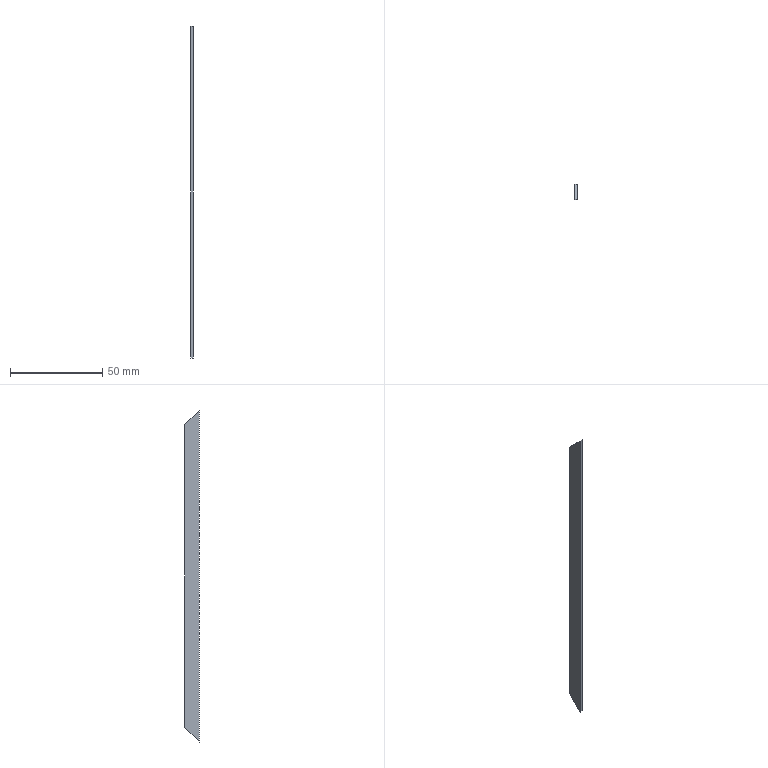Part | NX | features BREP 1 | 1 solid | 6 faces | box 1.5 x 8 x 179.5 mm | volume 2058 mm3 | plane 6
STEP:
#1=CARTESIAN_POINT('',(0.,8.,81.75));
#2=VERTEX_POINT('',#1);
#3=CARTESIAN_POINT('',(0.,8.,-81.75));
#4=VERTEX_POINT('',#3);
#5=CARTESIAN_POINT('',(0.,8.,89.75));
#6=DIRECTION('',(0.,0.,-1.));
#7=VECTOR('',#6,1000.);
#8=LINE('',#5,#7);
#9=EDGE_CURVE('',#2,#4,#8,.T.);
#10=ORIENTED_EDGE('',*,*,#9,.T.);
#11=CARTESIAN_POINT('',(0.,0.,-89.75));
#12=VERTEX_POINT('',#11);
#13=CARTESIAN_POINT('',(0.,8.,-81.75));
#14=DIRECTION('',(0.,-0.7071,-0.7071));
#15=VECTOR('',#14,1000.);
#16=LINE('',#13,#15);
#17=EDGE_CURVE('',#4,#12,#16,.T.);
#18=ORIENTED_EDGE('',*,*,#17,.T.);
#19=CARTESIAN_POINT('',(0.,0.,89.75));
#20=VERTEX_POINT('',#19);
#21=CARTESIAN_POINT('',(0.,0.,89.75));
#22=DIRECTION('',(0.,0.,-1.));
#23=VECTOR('',#22,1000.);
#24=LINE('',#21,#23);
#25=EDGE_CURVE('',#20,#12,#24,.T.);
#26=ORIENTED_EDGE('',*,*,#25,.F.);
#27=CARTESIAN_POINT('',(0.,0.,89.75));
#28=DIRECTION('',(0.,0.7071,-0.7071));
#29=VECTOR('',#28,1000.);
#30=LINE('',#27,#29);
#31=EDGE_CURVE('',#20,#2,#30,.T.);
#32=ORIENTED_EDGE('',*,*,#31,.T.);
#33=EDGE_LOOP('',(#10,#18,#26,#32));
#34=FACE_BOUND('',#33,.T.);
#35=CARTESIAN_POINT('',(0.,0.,89.75));
#36=DIRECTION('',(1.,0.,0.));
#37=DIRECTION('',(0.,1.,0.));
#38=AXIS2_PLACEMENT_3D('',#35,#36,#37);
#39=PLANE('',#38);
#40=ADVANCED_FACE('',(#34),#39,.F.);
#41=CARTESIAN_POINT('',(1.5,0.,-89.75));
#42=VERTEX_POINT('',#41);
#43=CARTESIAN_POINT('',(0.,0.,-89.75));
#44=DIRECTION('',(1.,0.,0.));
#45=VECTOR('',#44,1000.);
#46=LINE('',#43,#45);
#47=EDGE_CURVE('',#12,#42,#46,.T.);
#48=ORIENTED_EDGE('',*,*,#47,.T.);
#49=CARTESIAN_POINT('',(1.5,0.,89.75));
#50=VERTEX_POINT('',#49);
#51=CARTESIAN_POINT('',(1.5,0.,89.75));
#52=DIRECTION('',(0.,0.,-1.));
#53=VECTOR('',#52,1000.);
#54=LINE('',#51,#53);
#55=EDGE_CURVE('',#50,#42,#54,.T.);
#56=ORIENTED_EDGE('',*,*,#55,.F.);
#57=CARTESIAN_POINT('',(0.,0.,89.75));
#58=DIRECTION('',(1.,0.,0.));
#59=VECTOR('',#58,1000.);
#60=LINE('',#57,#59);
#61=EDGE_CURVE('',#20,#50,#60,.T.);
#62=ORIENTED_EDGE('',*,*,#61,.F.);
#63=ORIENTED_EDGE('',*,*,#25,.T.);
#64=EDGE_LOOP('',(#48,#56,#62,#63));
#65=FACE_BOUND('',#64,.T.);
#66=CARTESIAN_POINT('',(0.,0.,89.75));
#67=DIRECTION('',(0.,1.,0.));
#68=DIRECTION('',(1.,0.,0.));
#69=AXIS2_PLACEMENT_3D('',#66,#67,#68);
#70=PLANE('',#69);
#71=ADVANCED_FACE('',(#65),#70,.F.);
#72=ORIENTED_EDGE('',*,*,#55,.T.);
#73=CARTESIAN_POINT('',(1.5,8.,-81.75));
#74=VERTEX_POINT('',#73);
#75=CARTESIAN_POINT('',(1.5,8.,-81.75));
#76=DIRECTION('',(0.,0.7071,0.7071));
#77=VECTOR('',#76,1000.);
#78=LINE('',#75,#77);
#79=EDGE_CURVE('',#42,#74,#78,.T.);
#80=ORIENTED_EDGE('',*,*,#79,.T.);
#81=CARTESIAN_POINT('',(1.5,8.,81.75));
#82=VERTEX_POINT('',#81);
#83=CARTESIAN_POINT('',(1.5,8.,89.75));
#84=DIRECTION('',(0.,0.,-1.));
#85=VECTOR('',#84,1000.);
#86=LINE('',#83,#85);
#87=EDGE_CURVE('',#82,#74,#86,.T.);
#88=ORIENTED_EDGE('',*,*,#87,.F.);
#89=CARTESIAN_POINT('',(1.5,0.,89.75));
#90=DIRECTION('',(0.,-0.7071,0.7071));
#91=VECTOR('',#90,1000.);
#92=LINE('',#89,#91);
#93=EDGE_CURVE('',#82,#50,#92,.T.);
#94=ORIENTED_EDGE('',*,*,#93,.T.);
#95=EDGE_LOOP('',(#72,#80,#88,#94));
#96=FACE_BOUND('',#95,.T.);
#97=CARTESIAN_POINT('',(1.5,0.,89.75));
#98=DIRECTION('',(-1.,0.,0.));
#99=DIRECTION('',(0.,0.,1.));
#100=AXIS2_PLACEMENT_3D('',#97,#98,#99);
#101=PLANE('',#100);
#102=ADVANCED_FACE('',(#96),#101,.F.);
#103=ORIENTED_EDGE('',*,*,#87,.T.);
#104=CARTESIAN_POINT('',(0.,8.,-81.75));
#105=DIRECTION('',(-1.,0.,0.));
#106=VECTOR('',#105,1000.);
#107=LINE('',#104,#106);
#108=EDGE_CURVE('',#74,#4,#107,.T.);
#109=ORIENTED_EDGE('',*,*,#108,.T.);
#110=ORIENTED_EDGE('',*,*,#9,.F.);
#111=CARTESIAN_POINT('',(0.,8.,81.75));
#112=DIRECTION('',(1.,0.,0.));
#113=VECTOR('',#112,1000.);
#114=LINE('',#111,#113);
#115=EDGE_CURVE('',#2,#82,#114,.T.);
#116=ORIENTED_EDGE('',*,*,#115,.T.);
#117=EDGE_LOOP('',(#103,#109,#110,#116));
#118=FACE_BOUND('',#117,.T.);
#119=CARTESIAN_POINT('',(0.,8.,89.75));
#120=DIRECTION('',(0.,-1.,0.));
#121=DIRECTION('',(0.,0.,-1.));
#122=AXIS2_PLACEMENT_3D('',#119,#120,#121);
#123=PLANE('',#122);
#124=ADVANCED_FACE('',(#118),#123,.F.);
#125=ORIENTED_EDGE('',*,*,#79,.F.);
#126=ORIENTED_EDGE('',*,*,#47,.F.);
#127=ORIENTED_EDGE('',*,*,#17,.F.);
#128=ORIENTED_EDGE('',*,*,#108,.F.);
#129=EDGE_LOOP('',(#125,#126,#127,#128));
#130=FACE_BOUND('',#129,.T.);
#131=CARTESIAN_POINT('',(0.,8.,-81.75));
#132=DIRECTION('',(0.,0.7071,-0.7071));
#133=DIRECTION('',(-1.,0.,0.));
#134=AXIS2_PLACEMENT_3D('',#131,#132,#133);
#135=PLANE('',#134);
#136=ADVANCED_FACE('',(#130),#135,.T.);
#137=ORIENTED_EDGE('',*,*,#93,.F.);
#138=ORIENTED_EDGE('',*,*,#115,.F.);
#139=ORIENTED_EDGE('',*,*,#31,.F.);
#140=ORIENTED_EDGE('',*,*,#61,.T.);
#141=EDGE_LOOP('',(#137,#138,#139,#140));
#142=FACE_BOUND('',#141,.T.);
#143=CARTESIAN_POINT('',(0.,0.,89.75));
#144=DIRECTION('',(0.,-0.7071,-0.7071));
#145=DIRECTION('',(0.,0.7071,-0.7071));
#146=AXIS2_PLACEMENT_3D('',#143,#144,#145);
#147=PLANE('',#146);
#148=ADVANCED_FACE('',(#142),#147,.F.);
#149=CLOSED_SHELL('',(#40,#71,#102,#124,#136,#148));
#150=MANIFOLD_SOLID_BREP('',#149);
#151=(LENGTH_UNIT()NAMED_UNIT(*)SI_UNIT(.MILLI.,.METRE.));
#152=UNCERTAINTY_MEASURE_WITH_UNIT(LENGTH_MEASURE(0.00001),#151,'','');
#153=(NAMED_UNIT(*)PLANE_ANGLE_UNIT()SI_UNIT($,.RADIAN.));
#154=(NAMED_UNIT(*)SI_UNIT($,.STERADIAN.)SOLID_ANGLE_UNIT());
#155=(GEOMETRIC_REPRESENTATION_CONTEXT(3)GLOBAL_UNCERTAINTY_ASSIGNED_CONTEXT((#152))GLOBAL_UNIT_ASSIGNED_CONTEXT((#151,#153,#154))REPRESENTATION_CONTEXT('',''));
#156=ADVANCED_BREP_SHAPE_REPRESENTATION('',(#150),#155);